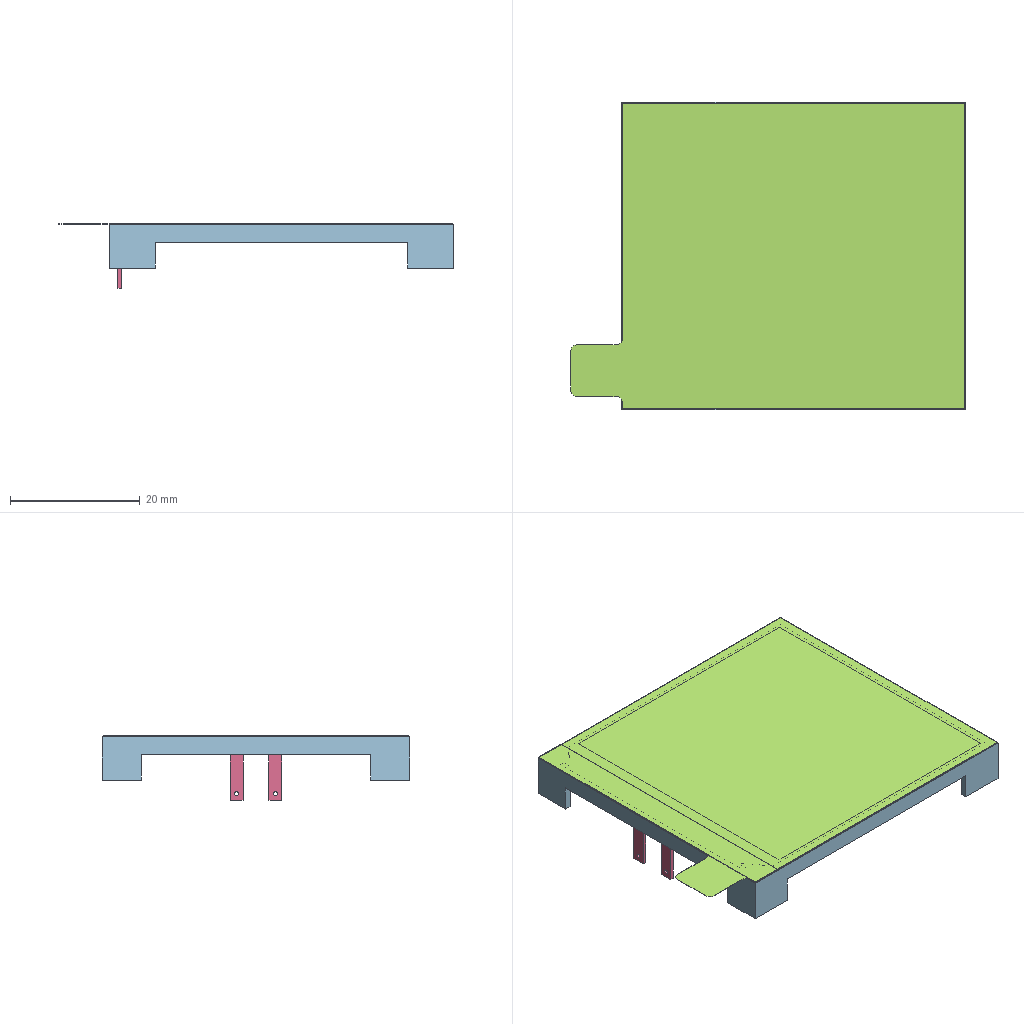Assembly | NX | 7 different items | 7 placed | box 61 x 47 x 10 mm
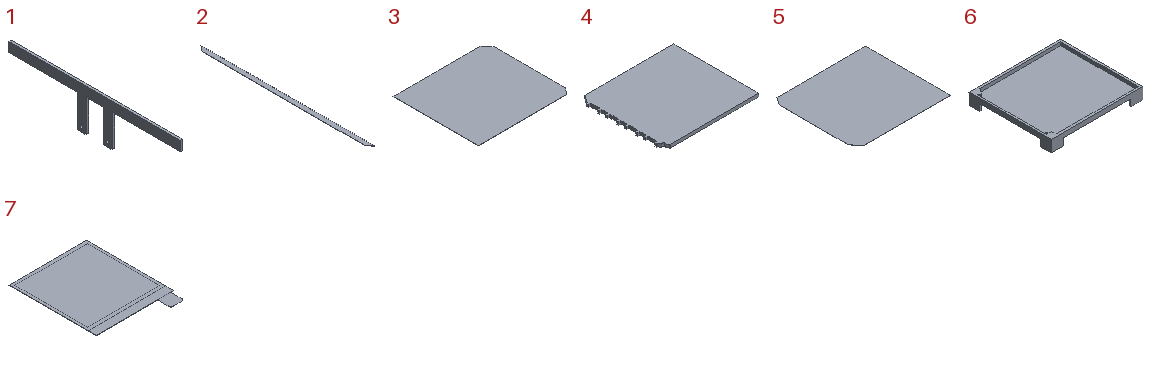Parts list (item | quantity | size | volume | features):
1 | x1 | 0.6 x 39.5 x 9.68 mm | 70.179 mm3 | features DATUM_CSYS 3, SIMPLE HOLE 2, SKETCH 2, EXTRUDE 1, HOLE PACKAGE 1
2 | x1 | 1 x 38.63 x 0.05 mm | 1.865 mm3 | features DATUM_CSYS 2, EXTRUDE 1, SKETCH 1
3 | x1 | 48.88 x 44.5 x 0.1 mm | 216.462 mm3 | features DATUM_CSYS 2, EXTRUDE 1, SKETCH 1
4 | x1 | 49.65 x 44.7 x 1.67 mm | 3632 mm3 | features DATUM_CSYS 3, SKETCH 2, BLEND 1, EXTRUDE 1, HOLE PACKAGE 1, SIMPLE HOLE 1
5 | x1 | 49.09 x 44.4 x 0.05 mm | 108.301 mm3 | features DATUM_CSYS 2, EXTRUDE 1, SKETCH 1
6 | x1 | 53 x 47.4 x 6.67 mm | 2471 mm3 | features DATUM_CSYS 6, EXTRUDE 5, SKETCH 5
7 | x1 | 47.2 x 60.8 x 0.18 mm | 184.569 mm3 | features DATUM_CSYS 6, EXTRUDE 6, SKETCH 5
Mates (type | each side: item.copy, entity, surface, feature):
Center22 | 1.1 face plane Extrude(1) | 1.1 face plane Extrude(1) | 6.1 face plane Extrude(5) | 6.1 face plane Extrude(5)
Touch | 1.1 face plane Extrude(1) | 6.1 face plane Extrude(4)
Touch | 1.1 face plane Extrude(1) | 6.1 face plane Extrude(3)
Fix | 6.1 component
Distance | 6.1 face plane Extrude(3) | 3.1 face plane Extrude(1)
Center22 | 6.1 face plane Extrude(3) | 6.1 face plane Extrude(3) | 3.1 edge | 3.1 edge
Touch | 3.1 edge | 6.1 face plane Extrude(3)
Center22 | 4.1 face plane Extrude(1) | 4.1 face plane Extrude(1) | 6.1 face plane Extrude(3) | 6.1 face plane Extrude(3)
Distance | 6.1 face plane Extrude(3) | 4.1 face plane Extrude(1)
Touch | 4.1 face plane Extrude(1) | 3.1 edge
Touch | 2.1 face plane Extrude(1) | 5.1 face plane Extrude(1)
Distance | 2.1 edge | 5.1 edge
Center22 | 5.1 edge | 5.1 edge | 4.1 edge | 6.1 edge
Center22 | 7.1 face plane Extrude(3) | 7.1 face plane Extrude(3) | 6.1 face plane Extrude(1) | 6.1 face plane Extrude(1)
Center22 | 6.1 face plane Extrude(1) | 6.1 face plane Extrude(1) | 7.1 face plane Extrude(3) | 7.1 face plane Extrude(3)
Touch | 7.1 face plane Extrude(3) | 6.1 face plane Extrude(1)
Distance | 7.1 face plane Extrude(3) | 5.1 face plane Extrude(1)